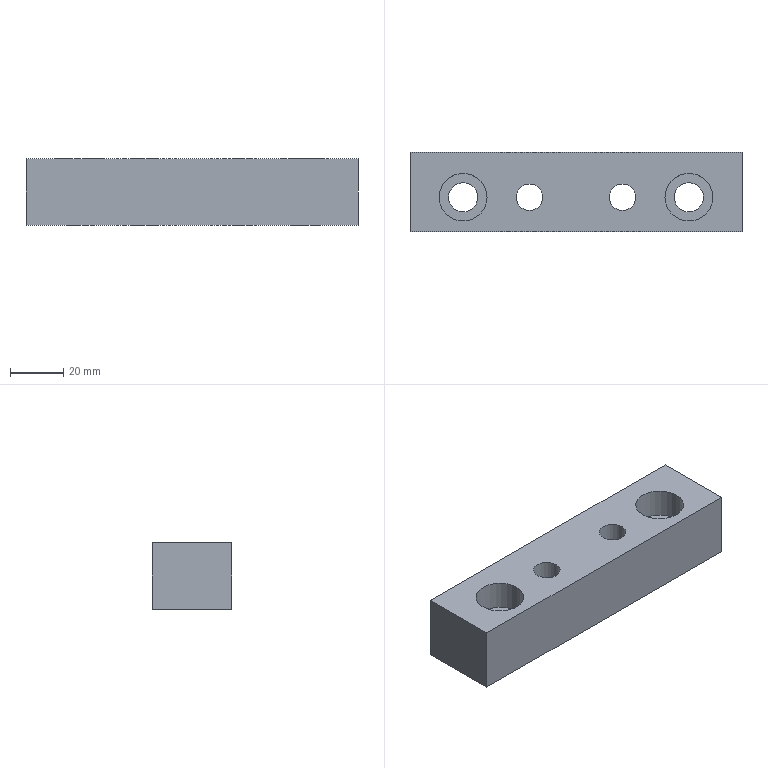Part | STEP file | solid 14 | 1 solid | 14 faces | box 125 x 30 x 25 mm | volume 81564 mm3 | plane 8 | cylinder 6 | commonest cylinder face diameters 10 x2 11 x2 18 x2